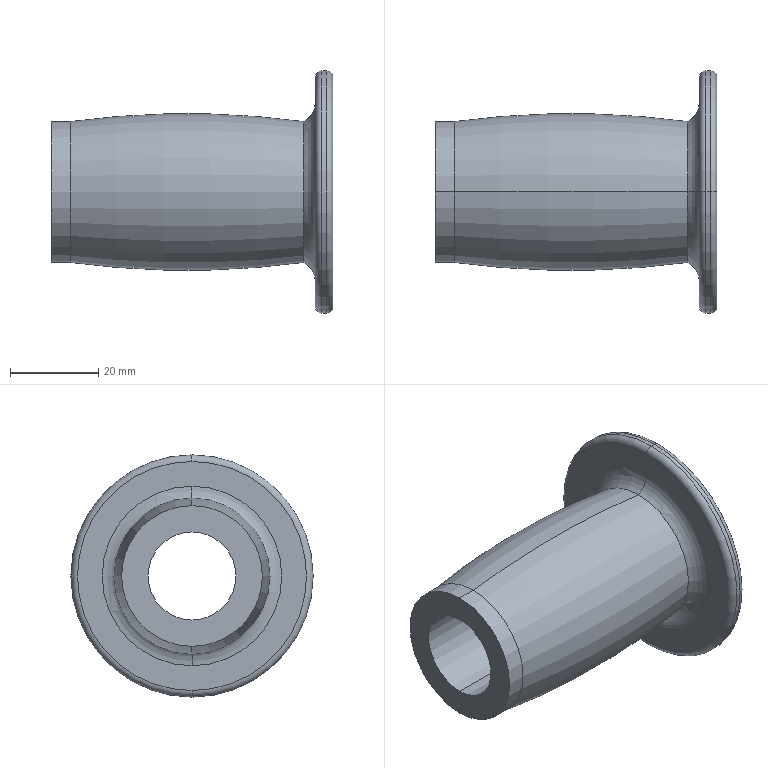Part | STEP file | Handlebar gear change grip | 1 solid | 17 faces | box 64 x 55 x 55 mm | volume 44472 mm3 | torus 6 | cylinder 6 | plane 3 | other 2 | commonest cylinder face diameters 20 x2 32 x2 55 x2
STEP:
#1=CARTESIAN_POINT('',(0.,0.,0.));
#2=DIRECTION('',(0.,0.,1.));
#3=DIRECTION('',(1.,0.,0.));
#4=AXIS2_PLACEMENT_3D('',#1,#2,#3);
#5=CARTESIAN_POINT('',(60.,0.,26.));
#6=VERTEX_POINT('',#5);
#7=CARTESIAN_POINT('',(60.,0.,-26.));
#8=VERTEX_POINT('',#7);
#9=CARTESIAN_POINT('',(60.,0.,0.));
#10=DIRECTION('',(-1.,0.,0.));
#11=DIRECTION('',(0.,0.,-1.));
#12=AXIS2_PLACEMENT_3D('',#9,#10,#11);
#13=CIRCLE('',#12,26.);
#14=CARTESIAN_POINT('',(61.5,0.,0.));
#15=DIRECTION('',(1.,0.,0.));
#16=DIRECTION('',(0.,0.,-1.));
#17=AXIS2_PLACEMENT_3D('',#14,#15,#16);
#18=TOROIDAL_SURFACE('',#17,26.,1.5);
#19=CARTESIAN_POINT('',(6.283,4.712));
#20=DIRECTION('',(-1.,0.));
#21=VECTOR('',#20,1.);
#22=LINE('',#19,#21);
#23=(GEOMETRIC_REPRESENTATION_CONTEXT(2)PARAMETRIC_REPRESENTATION_CONTEXT()REPRESENTATION_CONTEXT('',''));
#24=DEFINITIONAL_REPRESENTATION('',(#22),#23);
#25=PCURVE('',#18,#24);
#26=CARTESIAN_POINT('',(60.,0.,-16.));
#27=DIRECTION('',(1.,0.,0.));
#28=DIRECTION('',(0.,0.,-1.));
#29=AXIS2_PLACEMENT_3D('',#26,#27,#28);
#30=PLANE('',#29);
#31=CARTESIAN_POINT('',(10.,0.));
#32=CARTESIAN_POINT('',(10.,-45.033));
#33=CARTESIAN_POINT('',(-29.,-22.517));
#34=CARTESIAN_POINT('',(-68.,0.));
#35=CARTESIAN_POINT('',(-29.,22.517));
#36=CARTESIAN_POINT('',(10.,45.033));
#37=CARTESIAN_POINT('',(10.,0.));
#38=(BOUNDED_CURVE()B_SPLINE_CURVE(2,(#31,#32,#33,#34,#35,#36,#37),.UNSPECIFIED.,.T.,.F.)B_SPLINE_CURVE_WITH_KNOTS((1,2,2,2,2,1),(-2.094,0.,2.094,4.189,6.283,8.378),.UNSPECIFIED.)CURVE()GEOMETRIC_REPRESENTATION_ITEM()RATIONAL_B_SPLINE_CURVE((1.,0.5,1.,0.5,1.,0.5,1.))REPRESENTATION_ITEM(''));
#39=(GEOMETRIC_REPRESENTATION_CONTEXT(2)PARAMETRIC_REPRESENTATION_CONTEXT()REPRESENTATION_CONTEXT('',''));
#40=DEFINITIONAL_REPRESENTATION('',(#38),#39);
#41=PCURVE('',#30,#40);
#42=SURFACE_CURVE('',#13,(#25,#41),.PCURVE_S1.);
#43=EDGE_CURVE('',#6,#8,#42,.T.);
#44=ORIENTED_EDGE('',*,*,#43,.F.);
#45=CARTESIAN_POINT('',(61.5,0.,27.5));
#46=VERTEX_POINT('',#45);
#47=CARTESIAN_POINT('',(61.5,0.,26.));
#48=DIRECTION('',(0.,1.,0.));
#49=DIRECTION('',(0.,0.,1.));
#50=AXIS2_PLACEMENT_3D('',#47,#48,#49);
#51=CIRCLE('',#50,1.5);
#52=CARTESIAN_POINT('',(3.142,0.));
#53=DIRECTION('',(0.,1.));
#54=VECTOR('',#53,1.);
#55=LINE('',#52,#54);
#56=(GEOMETRIC_REPRESENTATION_CONTEXT(2)PARAMETRIC_REPRESENTATION_CONTEXT()REPRESENTATION_CONTEXT('',''));
#57=DEFINITIONAL_REPRESENTATION('',(#55),#56);
#58=PCURVE('',#18,#57);
#59=CARTESIAN_POINT('',(61.5,0.,0.));
#60=DIRECTION('',(1.,0.,0.));
#61=DIRECTION('',(0.,0.,-1.));
#62=AXIS2_PLACEMENT_3D('',#59,#60,#61);
#63=TOROIDAL_SURFACE('',#62,26.,1.5);
#64=CARTESIAN_POINT('',(3.142,0.));
#65=DIRECTION('',(0.,1.));
#66=VECTOR('',#65,1.);
#67=LINE('',#64,#66);
#68=(GEOMETRIC_REPRESENTATION_CONTEXT(2)PARAMETRIC_REPRESENTATION_CONTEXT()REPRESENTATION_CONTEXT('',''));
#69=DEFINITIONAL_REPRESENTATION('',(#67),#68);
#70=PCURVE('',#63,#69);
#71=SURFACE_CURVE('',#51,(#58,#70),.PCURVE_S1.);
#72=EDGE_CURVE('',#6,#46,#71,.T.);
#73=ORIENTED_EDGE('',*,*,#72,.T.);
#74=CARTESIAN_POINT('',(61.5,0.,-27.5));
#75=VERTEX_POINT('',#74);
#76=CARTESIAN_POINT('',(61.5,0.,0.));
#77=DIRECTION('',(1.,0.,0.));
#78=DIRECTION('',(0.,0.,-1.));
#79=AXIS2_PLACEMENT_3D('',#76,#77,#78);
#80=CIRCLE('',#79,27.5);
#81=CARTESIAN_POINT('',(0.,6.283));
#82=DIRECTION('',(1.,0.));
#83=VECTOR('',#82,1.);
#84=LINE('',#81,#83);
#85=(GEOMETRIC_REPRESENTATION_CONTEXT(2)PARAMETRIC_REPRESENTATION_CONTEXT()REPRESENTATION_CONTEXT('',''));
#86=DEFINITIONAL_REPRESENTATION('',(#84),#85);
#87=PCURVE('',#18,#86);
#88=CARTESIAN_POINT('',(64.,0.,0.));
#89=DIRECTION('',(-1.,0.,0.));
#90=DIRECTION('',(0.,0.,1.));
#91=AXIS2_PLACEMENT_3D('',#88,#89,#90);
#92=CYLINDRICAL_SURFACE('',#91,27.5);
#93=CARTESIAN_POINT('',(3.142,2.5));
#94=DIRECTION('',(-1.,0.));
#95=VECTOR('',#94,1.);
#96=LINE('',#93,#95);
#97=(GEOMETRIC_REPRESENTATION_CONTEXT(2)PARAMETRIC_REPRESENTATION_CONTEXT()REPRESENTATION_CONTEXT('',''));
#98=DEFINITIONAL_REPRESENTATION('',(#96),#97);
#99=PCURVE('',#92,#98);
#100=SURFACE_CURVE('',#80,(#87,#99),.PCURVE_S1.);
#101=EDGE_CURVE('',#75,#46,#100,.T.);
#102=ORIENTED_EDGE('',*,*,#101,.F.);
#103=CARTESIAN_POINT('',(61.5,0.,-26.));
#104=DIRECTION('',(0.,-1.,0.));
#105=DIRECTION('',(0.,0.,-1.));
#106=AXIS2_PLACEMENT_3D('',#103,#104,#105);
#107=CIRCLE('',#106,1.5);
#108=CARTESIAN_POINT('',(0.,0.));
#109=DIRECTION('',(0.,1.));
#110=VECTOR('',#109,1.);
#111=LINE('',#108,#110);
#112=(GEOMETRIC_REPRESENTATION_CONTEXT(2)PARAMETRIC_REPRESENTATION_CONTEXT()REPRESENTATION_CONTEXT('',''));
#113=DEFINITIONAL_REPRESENTATION('',(#111),#112);
#114=PCURVE('',#18,#113);
#115=CARTESIAN_POINT('',(6.283,0.));
#116=DIRECTION('',(0.,1.));
#117=VECTOR('',#116,1.);
#118=LINE('',#115,#117);
#119=(GEOMETRIC_REPRESENTATION_CONTEXT(2)PARAMETRIC_REPRESENTATION_CONTEXT()REPRESENTATION_CONTEXT('',''));
#120=DEFINITIONAL_REPRESENTATION('',(#118),#119);
#121=PCURVE('',#63,#120);
#122=SURFACE_CURVE('',#107,(#114,#121),.PCURVE_S1.);
#123=EDGE_CURVE('',#8,#75,#122,.T.);
#124=ORIENTED_EDGE('',*,*,#123,.F.);
#125=EDGE_LOOP('',(#44,#73,#102,#124));
#126=FACE_BOUND('',#125,.T.);
#127=ADVANCED_FACE('',(#126),#18,.T.);
#128=CARTESIAN_POINT('',(62.5,0.,27.5));
#129=VERTEX_POINT('',#128);
#130=CARTESIAN_POINT('',(62.5,0.,-27.5));
#131=VERTEX_POINT('',#130);
#132=CARTESIAN_POINT('',(62.5,0.,0.));
#133=DIRECTION('',(-1.,0.,0.));
#134=DIRECTION('',(0.,0.,1.));
#135=AXIS2_PLACEMENT_3D('',#132,#133,#134);
#136=CIRCLE('',#135,27.5);
#137=CARTESIAN_POINT('',(0.,1.5));
#138=DIRECTION('',(1.,0.));
#139=VECTOR('',#138,1.);
#140=LINE('',#137,#139);
#141=(GEOMETRIC_REPRESENTATION_CONTEXT(2)PARAMETRIC_REPRESENTATION_CONTEXT()REPRESENTATION_CONTEXT('',''));
#142=DEFINITIONAL_REPRESENTATION('',(#140),#141);
#143=PCURVE('',#92,#142);
#144=CARTESIAN_POINT('',(62.5,0.,0.));
#145=DIRECTION('',(-1.,0.,0.));
#146=DIRECTION('',(0.,0.,1.));
#147=AXIS2_PLACEMENT_3D('',#144,#145,#146);
#148=TOROIDAL_SURFACE('',#147,26.,1.5);
#149=CARTESIAN_POINT('',(0.,6.283));
#150=DIRECTION('',(1.,0.));
#151=VECTOR('',#150,1.);
#152=LINE('',#149,#151);
#153=(GEOMETRIC_REPRESENTATION_CONTEXT(2)PARAMETRIC_REPRESENTATION_CONTEXT()REPRESENTATION_CONTEXT('',''));
#154=DEFINITIONAL_REPRESENTATION('',(#152),#153);
#155=PCURVE('',#148,#154);
#156=SURFACE_CURVE('',#136,(#143,#155),.PCURVE_S1.);
#157=EDGE_CURVE('',#129,#131,#156,.T.);
#158=ORIENTED_EDGE('',*,*,#157,.T.);
#159=CARTESIAN_POINT('',(64.,0.,-27.5));
#160=DIRECTION('',(-1.,0.,0.));
#161=VECTOR('',#160,1.);
#162=LINE('',#159,#161);
#163=CARTESIAN_POINT('',(3.142,0.));
#164=DIRECTION('',(0.,1.));
#165=VECTOR('',#164,1.);
#166=LINE('',#163,#165);
#167=(GEOMETRIC_REPRESENTATION_CONTEXT(2)PARAMETRIC_REPRESENTATION_CONTEXT()REPRESENTATION_CONTEXT('',''));
#168=DEFINITIONAL_REPRESENTATION('',(#166),#167);
#169=PCURVE('',#92,#168);
#170=CARTESIAN_POINT('',(64.,0.,0.));
#171=DIRECTION('',(-1.,0.,0.));
#172=DIRECTION('',(0.,0.,1.));
#173=AXIS2_PLACEMENT_3D('',#170,#171,#172);
#174=CYLINDRICAL_SURFACE('',#173,27.5);
#175=CARTESIAN_POINT('',(3.142,0.));
#176=DIRECTION('',(0.,1.));
#177=VECTOR('',#176,1.);
#178=LINE('',#175,#177);
#179=(GEOMETRIC_REPRESENTATION_CONTEXT(2)PARAMETRIC_REPRESENTATION_CONTEXT()REPRESENTATION_CONTEXT('',''));
#180=DEFINITIONAL_REPRESENTATION('',(#178),#179);
#181=PCURVE('',#174,#180);
#182=SURFACE_CURVE('',#162,(#169,#181),.PCURVE_S1.);
#183=EDGE_CURVE('',#131,#75,#182,.T.);
#184=ORIENTED_EDGE('',*,*,#183,.T.);
#185=ORIENTED_EDGE('',*,*,#101,.T.);
#186=CARTESIAN_POINT('',(64.,0.,27.5));
#187=DIRECTION('',(-1.,0.,0.));
#188=VECTOR('',#187,1.);
#189=LINE('',#186,#188);
#190=CARTESIAN_POINT('',(0.,0.));
#191=DIRECTION('',(0.,1.));
#192=VECTOR('',#191,1.);
#193=LINE('',#190,#192);
#194=(GEOMETRIC_REPRESENTATION_CONTEXT(2)PARAMETRIC_REPRESENTATION_CONTEXT()REPRESENTATION_CONTEXT('',''));
#195=DEFINITIONAL_REPRESENTATION('',(#193),#194);
#196=PCURVE('',#92,#195);
#197=CARTESIAN_POINT('',(6.283,0.));
#198=DIRECTION('',(0.,1.));
#199=VECTOR('',#198,1.);
#200=LINE('',#197,#199);
#201=(GEOMETRIC_REPRESENTATION_CONTEXT(2)PARAMETRIC_REPRESENTATION_CONTEXT()REPRESENTATION_CONTEXT('',''));
#202=DEFINITIONAL_REPRESENTATION('',(#200),#201);
#203=PCURVE('',#174,#202);
#204=SURFACE_CURVE('',#189,(#196,#203),.PCURVE_S1.);
#205=EDGE_CURVE('',#129,#46,#204,.T.);
#206=ORIENTED_EDGE('',*,*,#205,.F.);
#207=EDGE_LOOP('',(#158,#184,#185,#206));
#208=FACE_BOUND('',#207,.T.);
#209=ADVANCED_FACE('',(#208),#92,.T.);
#210=ORIENTED_EDGE('',*,*,#183,.F.);
#211=CARTESIAN_POINT('',(62.5,0.,0.));
#212=DIRECTION('',(-1.,0.,0.));
#213=DIRECTION('',(0.,0.,1.));
#214=AXIS2_PLACEMENT_3D('',#211,#212,#213);
#215=CIRCLE('',#214,27.5);
#216=CARTESIAN_POINT('',(0.,1.5));
#217=DIRECTION('',(1.,0.));
#218=VECTOR('',#217,1.);
#219=LINE('',#216,#218);
#220=(GEOMETRIC_REPRESENTATION_CONTEXT(2)PARAMETRIC_REPRESENTATION_CONTEXT()REPRESENTATION_CONTEXT('',''));
#221=DEFINITIONAL_REPRESENTATION('',(#219),#220);
#222=PCURVE('',#174,#221);
#223=CARTESIAN_POINT('',(62.5,0.,0.));
#224=DIRECTION('',(-1.,0.,0.));
#225=DIRECTION('',(0.,0.,1.));
#226=AXIS2_PLACEMENT_3D('',#223,#224,#225);
#227=TOROIDAL_SURFACE('',#226,26.,1.5);
#228=CARTESIAN_POINT('',(0.,6.283));
#229=DIRECTION('',(1.,0.));
#230=VECTOR('',#229,1.);
#231=LINE('',#228,#230);
#232=(GEOMETRIC_REPRESENTATION_CONTEXT(2)PARAMETRIC_REPRESENTATION_CONTEXT()REPRESENTATION_CONTEXT('',''));
#233=DEFINITIONAL_REPRESENTATION('',(#231),#232);
#234=PCURVE('',#227,#233);
#235=SURFACE_CURVE('',#215,(#222,#234),.PCURVE_S1.);
#236=EDGE_CURVE('',#131,#129,#235,.T.);
#237=ORIENTED_EDGE('',*,*,#236,.T.);
#238=ORIENTED_EDGE('',*,*,#205,.T.);
#239=CARTESIAN_POINT('',(61.5,0.,0.));
#240=DIRECTION('',(1.,0.,0.));
#241=DIRECTION('',(0.,0.,-1.));
#242=AXIS2_PLACEMENT_3D('',#239,#240,#241);
#243=CIRCLE('',#242,27.5);
#244=CARTESIAN_POINT('',(9.425,2.5));
#245=DIRECTION('',(-1.,0.));
#246=VECTOR('',#245,1.);
#247=LINE('',#244,#246);
#248=(GEOMETRIC_REPRESENTATION_CONTEXT(2)PARAMETRIC_REPRESENTATION_CONTEXT()REPRESENTATION_CONTEXT('',''));
#249=DEFINITIONAL_REPRESENTATION('',(#247),#248);
#250=PCURVE('',#174,#249);
#251=CARTESIAN_POINT('',(0.,6.283));
#252=DIRECTION('',(1.,0.));
#253=VECTOR('',#252,1.);
#254=LINE('',#251,#253);
#255=(GEOMETRIC_REPRESENTATION_CONTEXT(2)PARAMETRIC_REPRESENTATION_CONTEXT()REPRESENTATION_CONTEXT('',''));
#256=DEFINITIONAL_REPRESENTATION('',(#254),#255);
#257=PCURVE('',#63,#256);
#258=SURFACE_CURVE('',#243,(#250,#257),.PCURVE_S1.);
#259=EDGE_CURVE('',#46,#75,#258,.T.);
#260=ORIENTED_EDGE('',*,*,#259,.T.);
#261=EDGE_LOOP('',(#210,#237,#238,#260));
#262=FACE_BOUND('',#261,.T.);
#263=ADVANCED_FACE('',(#262),#174,.T.);
#264=CARTESIAN_POINT('',(64.,0.,-26.));
#265=VERTEX_POINT('',#264);
#266=CARTESIAN_POINT('',(62.5,0.,-26.));
#267=DIRECTION('',(0.,1.,0.));
#268=DIRECTION('',(0.,0.,1.));
#269=AXIS2_PLACEMENT_3D('',#266,#267,#268);
#270=CIRCLE('',#269,1.5);
#271=CARTESIAN_POINT('',(3.142,3.142));
#272=DIRECTION('',(0.,1.));
#273=VECTOR('',#272,1.);
#274=LINE('',#271,#273);
#275=(GEOMETRIC_REPRESENTATION_CONTEXT(2)PARAMETRIC_REPRESENTATION_CONTEXT()REPRESENTATION_CONTEXT('',''));
#276=DEFINITIONAL_REPRESENTATION('',(#274),#275);
#277=PCURVE('',#227,#276);
#278=CARTESIAN_POINT('',(3.142,3.142));
#279=DIRECTION('',(0.,1.));
#280=VECTOR('',#279,1.);
#281=LINE('',#278,#280);
#282=(GEOMETRIC_REPRESENTATION_CONTEXT(2)PARAMETRIC_REPRESENTATION_CONTEXT()REPRESENTATION_CONTEXT('',''));
#283=DEFINITIONAL_REPRESENTATION('',(#281),#282);
#284=PCURVE('',#148,#283);
#285=SURFACE_CURVE('',#270,(#277,#284),.PCURVE_S1.);
#286=EDGE_CURVE('',#265,#131,#285,.T.);
#287=ORIENTED_EDGE('',*,*,#286,.F.);
#288=CARTESIAN_POINT('',(64.,0.,26.));
#289=VERTEX_POINT('',#288);
#290=CARTESIAN_POINT('',(64.,0.,0.));
#291=DIRECTION('',(1.,0.,0.));
#292=DIRECTION('',(0.,0.,1.));
#293=AXIS2_PLACEMENT_3D('',#290,#291,#292);
#294=CIRCLE('',#293,26.);
#295=CARTESIAN_POINT('',(6.283,4.712));
#296=DIRECTION('',(-1.,0.));
#297=VECTOR('',#296,1.);
#298=LINE('',#295,#297);
#299=(GEOMETRIC_REPRESENTATION_CONTEXT(2)PARAMETRIC_REPRESENTATION_CONTEXT()REPRESENTATION_CONTEXT('',''));
#300=DEFINITIONAL_REPRESENTATION('',(#298),#299);
#301=PCURVE('',#227,#300);
#302=CARTESIAN_POINT('',(64.,0.,-10.));
#303=DIRECTION('',(-1.,0.,0.));
#304=DIRECTION('',(0.,0.,1.));
#305=AXIS2_PLACEMENT_3D('',#302,#303,#304);
#306=PLANE('',#305);
#307=CARTESIAN_POINT('',(36.,0.));
#308=CARTESIAN_POINT('',(36.,-45.033));
#309=CARTESIAN_POINT('',(-3.,-22.517));
#310=CARTESIAN_POINT('',(-42.,0.));
#311=CARTESIAN_POINT('',(-3.,22.517));
#312=CARTESIAN_POINT('',(36.,45.033));
#313=CARTESIAN_POINT('',(36.,0.));
#314=(BOUNDED_CURVE()B_SPLINE_CURVE(2,(#307,#308,#309,#310,#311,#312,#313),.UNSPECIFIED.,.T.,.F.)B_SPLINE_CURVE_WITH_KNOTS((1,2,2,2,2,1),(-2.094,0.,2.094,4.189,6.283,8.378),.UNSPECIFIED.)CURVE()GEOMETRIC_REPRESENTATION_ITEM()RATIONAL_B_SPLINE_CURVE((1.,0.5,1.,0.5,1.,0.5,1.))REPRESENTATION_ITEM(''));
#315=(GEOMETRIC_REPRESENTATION_CONTEXT(2)PARAMETRIC_REPRESENTATION_CONTEXT()REPRESENTATION_CONTEXT('',''));
#316=DEFINITIONAL_REPRESENTATION('',(#314),#315);
#317=PCURVE('',#306,#316);
#318=SURFACE_CURVE('',#294,(#301,#317),.PCURVE_S1.);
#319=EDGE_CURVE('',#289,#265,#318,.T.);
#320=ORIENTED_EDGE('',*,*,#319,.F.);
#321=CARTESIAN_POINT('',(62.5,0.,26.));
#322=DIRECTION('',(0.,-1.,0.));
#323=DIRECTION('',(0.,0.,-1.));
#324=AXIS2_PLACEMENT_3D('',#321,#322,#323);
#325=CIRCLE('',#324,1.5);
#326=CARTESIAN_POINT('',(6.283,3.142));
#327=DIRECTION('',(0.,1.));
#328=VECTOR('',#327,1.);
#329=LINE('',#326,#328);
#330=(GEOMETRIC_REPRESENTATION_CONTEXT(2)PARAMETRIC_REPRESENTATION_CONTEXT()REPRESENTATION_CONTEXT('',''));
#331=DEFINITIONAL_REPRESENTATION('',(#329),#330);
#332=PCURVE('',#227,#331);
#333=CARTESIAN_POINT('',(0.,3.142));
#334=DIRECTION('',(0.,1.));
#335=VECTOR('',#334,1.);
#336=LINE('',#333,#335);
#337=(GEOMETRIC_REPRESENTATION_CONTEXT(2)PARAMETRIC_REPRESENTATION_CONTEXT()REPRESENTATION_CONTEXT('',''));
#338=DEFINITIONAL_REPRESENTATION('',(#336),#337);
#339=PCURVE('',#148,#338);
#340=SURFACE_CURVE('',#325,(#332,#339),.PCURVE_S1.);
#341=EDGE_CURVE('',#289,#129,#340,.T.);
#342=ORIENTED_EDGE('',*,*,#341,.T.);
#343=ORIENTED_EDGE('',*,*,#236,.F.);
#344=EDGE_LOOP('',(#287,#320,#342,#343));
#345=FACE_BOUND('',#344,.T.);
#346=ADVANCED_FACE('',(#345),#227,.T.);
#347=ORIENTED_EDGE('',*,*,#319,.T.);
#348=CARTESIAN_POINT('',(64.,0.,0.));
#349=DIRECTION('',(1.,0.,0.));
#350=DIRECTION('',(0.,0.,1.));
#351=AXIS2_PLACEMENT_3D('',#348,#349,#350);
#352=CIRCLE('',#351,26.);
#353=CARTESIAN_POINT('',(36.,0.));
#354=CARTESIAN_POINT('',(36.,-45.033));
#355=CARTESIAN_POINT('',(-3.,-22.517));
#356=CARTESIAN_POINT('',(-42.,0.));
#357=CARTESIAN_POINT('',(-3.,22.517));
#358=CARTESIAN_POINT('',(36.,45.033));
#359=CARTESIAN_POINT('',(36.,0.));
#360=(BOUNDED_CURVE()B_SPLINE_CURVE(2,(#353,#354,#355,#356,#357,#358,#359),.UNSPECIFIED.,.T.,.F.)B_SPLINE_CURVE_WITH_KNOTS((1,2,2,2,2,1),(-2.094,0.,2.094,4.189,6.283,8.378),.UNSPECIFIED.)CURVE()GEOMETRIC_REPRESENTATION_ITEM()RATIONAL_B_SPLINE_CURVE((1.,0.5,1.,0.5,1.,0.5,1.))REPRESENTATION_ITEM(''));
#361=(GEOMETRIC_REPRESENTATION_CONTEXT(2)PARAMETRIC_REPRESENTATION_CONTEXT()REPRESENTATION_CONTEXT('',''));
#362=DEFINITIONAL_REPRESENTATION('',(#360),#361);
#363=PCURVE('',#306,#362);
#364=CARTESIAN_POINT('',(6.283,4.712));
#365=DIRECTION('',(-1.,0.));
#366=VECTOR('',#365,1.);
#367=LINE('',#364,#366);
#368=(GEOMETRIC_REPRESENTATION_CONTEXT(2)PARAMETRIC_REPRESENTATION_CONTEXT()REPRESENTATION_CONTEXT('',''));
#369=DEFINITIONAL_REPRESENTATION('',(#367),#368);
#370=PCURVE('',#148,#369);
#371=SURFACE_CURVE('',#352,(#363,#370),.PCURVE_S1.);
#372=EDGE_CURVE('',#265,#289,#371,.T.);
#373=ORIENTED_EDGE('',*,*,#372,.T.);
#374=EDGE_LOOP('',(#347,#373));
#375=FACE_BOUND('',#374,.T.);
#376=CARTESIAN_POINT('',(64.,0.,10.));
#377=VERTEX_POINT('',#376);
#378=CARTESIAN_POINT('',(64.,0.,-10.));
#379=VERTEX_POINT('',#378);
#380=CARTESIAN_POINT('',(64.,0.,0.));
#381=DIRECTION('',(-1.,0.,0.));
#382=DIRECTION('',(0.,0.,1.));
#383=AXIS2_PLACEMENT_3D('',#380,#381,#382);
#384=CIRCLE('',#383,10.);
#385=CARTESIAN_POINT('',(10.,0.));
#386=DIRECTION('',(1.,0.));
#387=AXIS2_PLACEMENT_2D('',#385,#386);
#388=CIRCLE('',#387,10.);
#389=(GEOMETRIC_REPRESENTATION_CONTEXT(2)PARAMETRIC_REPRESENTATION_CONTEXT()REPRESENTATION_CONTEXT('',''));
#390=DEFINITIONAL_REPRESENTATION('',(#388),#389);
#391=PCURVE('',#306,#390);
#392=CARTESIAN_POINT('',(64.,0.,0.));
#393=DIRECTION('',(-1.,0.,0.));
#394=DIRECTION('',(0.,0.,1.));
#395=AXIS2_PLACEMENT_3D('',#392,#393,#394);
#396=CYLINDRICAL_SURFACE('',#395,10.);
#397=CARTESIAN_POINT('',(0.,0.));
#398=DIRECTION('',(1.,0.));
#399=VECTOR('',#398,1.);
#400=LINE('',#397,#399);
#401=(GEOMETRIC_REPRESENTATION_CONTEXT(2)PARAMETRIC_REPRESENTATION_CONTEXT()REPRESENTATION_CONTEXT('',''));
#402=DEFINITIONAL_REPRESENTATION('',(#400),#401);
#403=PCURVE('',#396,#402);
#404=SURFACE_CURVE('',#384,(#391,#403),.PCURVE_S1.);
#405=EDGE_CURVE('',#377,#379,#404,.T.);
#406=ORIENTED_EDGE('',*,*,#405,.T.);
#407=CARTESIAN_POINT('',(64.,0.,0.));
#408=DIRECTION('',(-1.,0.,0.));
#409=DIRECTION('',(0.,0.,1.));
#410=AXIS2_PLACEMENT_3D('',#407,#408,#409);
#411=CIRCLE('',#410,10.);
#412=CARTESIAN_POINT('',(10.,0.));
#413=DIRECTION('',(1.,0.));
#414=AXIS2_PLACEMENT_2D('',#412,#413);
#415=CIRCLE('',#414,10.);
#416=(GEOMETRIC_REPRESENTATION_CONTEXT(2)PARAMETRIC_REPRESENTATION_CONTEXT()REPRESENTATION_CONTEXT('',''));
#417=DEFINITIONAL_REPRESENTATION('',(#415),#416);
#418=PCURVE('',#306,#417);
#419=CARTESIAN_POINT('',(64.,0.,0.));
#420=DIRECTION('',(-1.,0.,0.));
#421=DIRECTION('',(0.,0.,1.));
#422=AXIS2_PLACEMENT_3D('',#419,#420,#421);
#423=CYLINDRICAL_SURFACE('',#422,10.);
#424=CARTESIAN_POINT('',(0.,0.));
#425=DIRECTION('',(1.,0.));
#426=VECTOR('',#425,1.);
#427=LINE('',#424,#426);
#428=(GEOMETRIC_REPRESENTATION_CONTEXT(2)PARAMETRIC_REPRESENTATION_CONTEXT()REPRESENTATION_CONTEXT('',''));
#429=DEFINITIONAL_REPRESENTATION('',(#427),#428);
#430=PCURVE('',#423,#429);
#431=SURFACE_CURVE('',#411,(#418,#430),.PCURVE_S1.);
#432=EDGE_CURVE('',#379,#377,#431,.T.);
#433=ORIENTED_EDGE('',*,*,#432,.T.);
#434=EDGE_LOOP('',(#406,#433));
#435=FACE_BOUND('',#434,.T.);
#436=ADVANCED_FACE('',(#375,#435),#306,.F.);
#437=CARTESIAN_POINT('',(0.,0.,10.));
#438=VERTEX_POINT('',#437);
#439=CARTESIAN_POINT('',(64.,0.,10.));
#440=DIRECTION('',(-1.,0.,0.));
#441=VECTOR('',#440,1.);
#442=LINE('',#439,#441);
#443=CARTESIAN_POINT('',(6.283,0.));
#444=DIRECTION('',(0.,1.));
#445=VECTOR('',#444,1.);
#446=LINE('',#443,#445);
#447=(GEOMETRIC_REPRESENTATION_CONTEXT(2)PARAMETRIC_REPRESENTATION_CONTEXT()REPRESENTATION_CONTEXT('',''));
#448=DEFINITIONAL_REPRESENTATION('',(#446),#447);
#449=PCURVE('',#423,#448);
#450=CARTESIAN_POINT('',(0.,0.));
#451=DIRECTION('',(0.,1.));
#452=VECTOR('',#451,1.);
#453=LINE('',#450,#452);
#454=(GEOMETRIC_REPRESENTATION_CONTEXT(2)PARAMETRIC_REPRESENTATION_CONTEXT()REPRESENTATION_CONTEXT('',''));
#455=DEFINITIONAL_REPRESENTATION('',(#453),#454);
#456=PCURVE('',#396,#455);
#457=SURFACE_CURVE('',#442,(#449,#456),.PCURVE_S1.);
#458=EDGE_CURVE('',#377,#438,#457,.T.);
#459=ORIENTED_EDGE('',*,*,#458,.T.);
#460=CARTESIAN_POINT('',(0.,0.,-10.));
#461=VERTEX_POINT('',#460);
#462=CARTESIAN_POINT('',(0.,0.,0.));
#463=DIRECTION('',(-1.,0.,0.));
#464=DIRECTION('',(0.,0.,1.));
#465=AXIS2_PLACEMENT_3D('',#462,#463,#464);
#466=CIRCLE('',#465,10.);
#467=CARTESIAN_POINT('',(0.,64.));
#468=DIRECTION('',(1.,0.));
#469=VECTOR('',#468,1.);
#470=LINE('',#467,#469);
#471=(GEOMETRIC_REPRESENTATION_CONTEXT(2)PARAMETRIC_REPRESENTATION_CONTEXT()REPRESENTATION_CONTEXT('',''));
#472=DEFINITIONAL_REPRESENTATION('',(#470),#471);
#473=PCURVE('',#423,#472);
#474=CARTESIAN_POINT('',(0.,0.,-10.));
#475=DIRECTION('',(1.,0.,0.));
#476=DIRECTION('',(0.,0.,-1.));
#477=AXIS2_PLACEMENT_3D('',#474,#475,#476);
#478=PLANE('',#477);
#479=CARTESIAN_POINT('',(-20.,0.));
#480=CARTESIAN_POINT('',(-20.,17.321));
#481=CARTESIAN_POINT('',(-5.,8.66));
#482=CARTESIAN_POINT('',(10.,0.));
#483=CARTESIAN_POINT('',(-5.,-8.66));
#484=CARTESIAN_POINT('',(-20.,-17.321));
#485=CARTESIAN_POINT('',(-20.,0.));
#486=(BOUNDED_CURVE()B_SPLINE_CURVE(2,(#479,#480,#481,#482,#483,#484,#485),.UNSPECIFIED.,.T.,.F.)B_SPLINE_CURVE_WITH_KNOTS((1,2,2,2,2,1),(-2.094,0.,2.094,4.189,6.283,8.378),.UNSPECIFIED.)CURVE()GEOMETRIC_REPRESENTATION_ITEM()RATIONAL_B_SPLINE_CURVE((1.,0.5,1.,0.5,1.,0.5,1.))REPRESENTATION_ITEM(''));
#487=(GEOMETRIC_REPRESENTATION_CONTEXT(2)PARAMETRIC_REPRESENTATION_CONTEXT()REPRESENTATION_CONTEXT('',''));
#488=DEFINITIONAL_REPRESENTATION('',(#486),#487);
#489=PCURVE('',#478,#488);
#490=SURFACE_CURVE('',#466,(#473,#489),.PCURVE_S1.);
#491=EDGE_CURVE('',#461,#438,#490,.T.);
#492=ORIENTED_EDGE('',*,*,#491,.F.);
#493=CARTESIAN_POINT('',(64.,0.,-10.));
#494=DIRECTION('',(-1.,0.,0.));
#495=VECTOR('',#494,1.);
#496=LINE('',#493,#495);
#497=CARTESIAN_POINT('',(3.142,0.));
#498=DIRECTION('',(0.,1.));
#499=VECTOR('',#498,1.);
#500=LINE('',#497,#499);
#501=(GEOMETRIC_REPRESENTATION_CONTEXT(2)PARAMETRIC_REPRESENTATION_CONTEXT()REPRESENTATION_CONTEXT('',''));
#502=DEFINITIONAL_REPRESENTATION('',(#500),#501);
#503=PCURVE('',#423,#502);
#504=CARTESIAN_POINT('',(3.142,0.));
#505=DIRECTION('',(0.,1.));
#506=VECTOR('',#505,1.);
#507=LINE('',#504,#506);
#508=(GEOMETRIC_REPRESENTATION_CONTEXT(2)PARAMETRIC_REPRESENTATION_CONTEXT()REPRESENTATION_CONTEXT('',''));
#509=DEFINITIONAL_REPRESENTATION('',(#507),#508);
#510=PCURVE('',#396,#509);
#511=SURFACE_CURVE('',#496,(#503,#510),.PCURVE_S1.);
#512=EDGE_CURVE('',#379,#461,#511,.T.);
#513=ORIENTED_EDGE('',*,*,#512,.F.);
#514=ORIENTED_EDGE('',*,*,#432,.T.);
#515=EDGE_LOOP('',(#459,#492,#513,#514));
#516=FACE_BOUND('',#515,.F.);
#517=ADVANCED_FACE('',(#516),#423,.F.);
#518=CARTESIAN_POINT('',(0.,0.,0.));
#519=DIRECTION('',(-1.,0.,0.));
#520=DIRECTION('',(0.,0.,1.));
#521=AXIS2_PLACEMENT_3D('',#518,#519,#520);
#522=CIRCLE('',#521,10.);
#523=CARTESIAN_POINT('',(-20.,0.));
#524=CARTESIAN_POINT('',(-20.,17.321));
#525=CARTESIAN_POINT('',(-5.,8.66));
#526=CARTESIAN_POINT('',(10.,0.));
#527=CARTESIAN_POINT('',(-5.,-8.66));
#528=CARTESIAN_POINT('',(-20.,-17.321));
#529=CARTESIAN_POINT('',(-20.,0.));
#530=(BOUNDED_CURVE()B_SPLINE_CURVE(2,(#523,#524,#525,#526,#527,#528,#529),.UNSPECIFIED.,.T.,.F.)B_SPLINE_CURVE_WITH_KNOTS((1,2,2,2,2,1),(-2.094,0.,2.094,4.189,6.283,8.378),.UNSPECIFIED.)CURVE()GEOMETRIC_REPRESENTATION_ITEM()RATIONAL_B_SPLINE_CURVE((1.,0.5,1.,0.5,1.,0.5,1.))REPRESENTATION_ITEM(''));
#531=(GEOMETRIC_REPRESENTATION_CONTEXT(2)PARAMETRIC_REPRESENTATION_CONTEXT()REPRESENTATION_CONTEXT('',''));
#532=DEFINITIONAL_REPRESENTATION('',(#530),#531);
#533=PCURVE('',#478,#532);
#534=CARTESIAN_POINT('',(0.,64.));
#535=DIRECTION('',(1.,0.));
#536=VECTOR('',#535,1.);
#537=LINE('',#534,#536);
#538=(GEOMETRIC_REPRESENTATION_CONTEXT(2)PARAMETRIC_REPRESENTATION_CONTEXT()REPRESENTATION_CONTEXT('',''));
#539=DEFINITIONAL_REPRESENTATION('',(#537),#538);
#540=PCURVE('',#396,#539);
#541=SURFACE_CURVE('',#522,(#533,#540),.PCURVE_S1.);
#542=EDGE_CURVE('',#438,#461,#541,.T.);
#543=ORIENTED_EDGE('',*,*,#542,.F.);
#544=ORIENTED_EDGE('',*,*,#491,.F.);
#545=EDGE_LOOP('',(#543,#544));
#546=FACE_BOUND('',#545,.T.);
#547=CARTESIAN_POINT('',(0.,0.,16.));
#548=VERTEX_POINT('',#547);
#549=CARTESIAN_POINT('',(0.,0.,-16.));
#550=VERTEX_POINT('',#549);
#551=CARTESIAN_POINT('',(0.,0.,0.));
#552=DIRECTION('',(-1.,0.,0.));
#553=DIRECTION('',(0.,0.,1.));
#554=AXIS2_PLACEMENT_3D('',#551,#552,#553);
#555=CIRCLE('',#554,16.);
#556=CARTESIAN_POINT('',(-26.,0.));
#557=CARTESIAN_POINT('',(-26.,27.713));
#558=CARTESIAN_POINT('',(-2.,13.856));
#559=CARTESIAN_POINT('',(22.,0.));
#560=CARTESIAN_POINT('',(-2.,-13.856));
#561=CARTESIAN_POINT('',(-26.,-27.713));
#562=CARTESIAN_POINT('',(-26.,0.));
#563=(BOUNDED_CURVE()B_SPLINE_CURVE(2,(#556,#557,#558,#559,#560,#561,#562),.UNSPECIFIED.,.T.,.F.)B_SPLINE_CURVE_WITH_KNOTS((1,2,2,2,2,1),(-2.094,0.,2.094,4.189,6.283,8.378),.UNSPECIFIED.)CURVE()GEOMETRIC_REPRESENTATION_ITEM()RATIONAL_B_SPLINE_CURVE((1.,0.5,1.,0.5,1.,0.5,1.))REPRESENTATION_ITEM(''));
#564=(GEOMETRIC_REPRESENTATION_CONTEXT(2)PARAMETRIC_REPRESENTATION_CONTEXT()REPRESENTATION_CONTEXT('',''));
#565=DEFINITIONAL_REPRESENTATION('',(#563),#564);
#566=PCURVE('',#478,#565);
#567=CARTESIAN_POINT('',(64.,0.,0.));
#568=DIRECTION('',(-1.,0.,0.));
#569=DIRECTION('',(0.,0.,1.));
#570=AXIS2_PLACEMENT_3D('',#567,#568,#569);
#571=CYLINDRICAL_SURFACE('',#570,16.);
#572=CARTESIAN_POINT('',(0.,64.));
#573=DIRECTION('',(1.,0.));
#574=VECTOR('',#573,1.);
#575=LINE('',#572,#574);
#576=(GEOMETRIC_REPRESENTATION_CONTEXT(2)PARAMETRIC_REPRESENTATION_CONTEXT()REPRESENTATION_CONTEXT('',''));
#577=DEFINITIONAL_REPRESENTATION('',(#575),#576);
#578=PCURVE('',#571,#577);
#579=SURFACE_CURVE('',#555,(#566,#578),.PCURVE_S1.);
#580=EDGE_CURVE('',#548,#550,#579,.T.);
#581=ORIENTED_EDGE('',*,*,#580,.T.);
#582=CARTESIAN_POINT('',(0.,0.,0.));
#583=DIRECTION('',(-1.,0.,0.));
#584=DIRECTION('',(0.,0.,1.));
#585=AXIS2_PLACEMENT_3D('',#582,#583,#584);
#586=CIRCLE('',#585,16.);
#587=CARTESIAN_POINT('',(-26.,0.));
#588=CARTESIAN_POINT('',(-26.,27.713));
#589=CARTESIAN_POINT('',(-2.,13.856));
#590=CARTESIAN_POINT('',(22.,0.));
#591=CARTESIAN_POINT('',(-2.,-13.856));
#592=CARTESIAN_POINT('',(-26.,-27.713));
#593=CARTESIAN_POINT('',(-26.,0.));
#594=(BOUNDED_CURVE()B_SPLINE_CURVE(2,(#587,#588,#589,#590,#591,#592,#593),.UNSPECIFIED.,.T.,.F.)B_SPLINE_CURVE_WITH_KNOTS((1,2,2,2,2,1),(-2.094,0.,2.094,4.189,6.283,8.378),.UNSPECIFIED.)CURVE()GEOMETRIC_REPRESENTATION_ITEM()RATIONAL_B_SPLINE_CURVE((1.,0.5,1.,0.5,1.,0.5,1.))REPRESENTATION_ITEM(''));
#595=(GEOMETRIC_REPRESENTATION_CONTEXT(2)PARAMETRIC_REPRESENTATION_CONTEXT()REPRESENTATION_CONTEXT('',''));
#596=DEFINITIONAL_REPRESENTATION('',(#594),#595);
#597=PCURVE('',#478,#596);
#598=CARTESIAN_POINT('',(64.,0.,0.));
#599=DIRECTION('',(-1.,0.,0.));
#600=DIRECTION('',(0.,0.,1.));
#601=AXIS2_PLACEMENT_3D('',#598,#599,#600);
#602=CYLINDRICAL_SURFACE('',#601,16.);
#603=CARTESIAN_POINT('',(0.,64.));
#604=DIRECTION('',(1.,0.));
#605=VECTOR('',#604,1.);
#606=LINE('',#603,#605);
#607=(GEOMETRIC_REPRESENTATION_CONTEXT(2)PARAMETRIC_REPRESENTATION_CONTEXT()REPRESENTATION_CONTEXT('',''));
#608=DEFINITIONAL_REPRESENTATION('',(#606),#607);
#609=PCURVE('',#602,#608);
#610=SURFACE_CURVE('',#586,(#597,#609),.PCURVE_S1.);
#611=EDGE_CURVE('',#550,#548,#610,.T.);
#612=ORIENTED_EDGE('',*,*,#611,.T.);
#613=EDGE_LOOP('',(#581,#612));
#614=FACE_BOUND('',#613,.T.);
#615=ADVANCED_FACE('',(#546,#614),#478,.F.);
#616=CARTESIAN_POINT('',(4.315,0.,-16.));
#617=VERTEX_POINT('',#616);
#618=CARTESIAN_POINT('',(64.,0.,-16.));
#619=DIRECTION('',(-1.,0.,0.));
#620=VECTOR('',#619,1.);
#621=LINE('',#618,#620);
#622=CARTESIAN_POINT('',(3.142,0.));
#623=DIRECTION('',(0.,1.));
#624=VECTOR('',#623,1.);
#625=LINE('',#622,#624);
#626=(GEOMETRIC_REPRESENTATION_CONTEXT(2)PARAMETRIC_REPRESENTATION_CONTEXT()REPRESENTATION_CONTEXT('',''));
#627=DEFINITIONAL_REPRESENTATION('',(#625),#626);
#628=PCURVE('',#602,#627);
#629=CARTESIAN_POINT('',(3.142,0.));
#630=DIRECTION('',(0.,1.));
#631=VECTOR('',#630,1.);
#632=LINE('',#629,#631);
#633=(GEOMETRIC_REPRESENTATION_CONTEXT(2)PARAMETRIC_REPRESENTATION_CONTEXT()REPRESENTATION_CONTEXT('',''));
#634=DEFINITIONAL_REPRESENTATION('',(#632),#633);
#635=PCURVE('',#571,#634);
#636=SURFACE_CURVE('',#621,(#628,#635),.PCURVE_S1.);
#637=EDGE_CURVE('',#617,#550,#636,.T.);
#638=ORIENTED_EDGE('',*,*,#637,.F.);
#639=CARTESIAN_POINT('',(4.315,0.,16.));
#640=VERTEX_POINT('',#639);
#641=CARTESIAN_POINT('',(4.315,0.,0.));
#642=DIRECTION('',(-1.,0.,0.));
#643=DIRECTION('',(0.,0.,1.));
#644=AXIS2_PLACEMENT_3D('',#641,#642,#643);
#645=CIRCLE('',#644,16.);
#646=CARTESIAN_POINT('',(0.,59.685));
#647=DIRECTION('',(1.,0.));
#648=VECTOR('',#647,1.);
#649=LINE('',#646,#648);
#650=(GEOMETRIC_REPRESENTATION_CONTEXT(2)PARAMETRIC_REPRESENTATION_CONTEXT()REPRESENTATION_CONTEXT('',''));
#651=DEFINITIONAL_REPRESENTATION('',(#649),#650);
#652=PCURVE('',#602,#651);
#653=CARTESIAN_POINT('',(4.315,0.,-16.));
#654=CARTESIAN_POINT('',(14.868,0.,-17.424));
#655=CARTESIAN_POINT('',(25.518,0.,-18.141));
#656=CARTESIAN_POINT('',(36.199,0.,-18.141));
#657=CARTESIAN_POINT('',(46.848,0.,-17.424));
#658=CARTESIAN_POINT('',(57.402,0.,-16.));
#659=B_SPLINE_CURVE_WITH_KNOTS('',5,(#653,#654,#655,#656,#657,#658),.UNSPECIFIED.,.F.,.F.,(6,6),(3.007,3.276),.PIECEWISE_BEZIER_KNOTS.);
#660=CARTESIAN_POINT('',(30.858,0.,0.));
#661=DIRECTION('',(-1.,0.,0.));
#662=AXIS1_PLACEMENT('',#660,#661);
#663=SURFACE_OF_REVOLUTION('',#659,#662);
#664=CARTESIAN_POINT('',(-3.142,3.007));
#665=DIRECTION('',(1.,0.));
#666=VECTOR('',#665,1.);
#667=LINE('',#664,#666);
#668=(GEOMETRIC_REPRESENTATION_CONTEXT(2)PARAMETRIC_REPRESENTATION_CONTEXT()REPRESENTATION_CONTEXT('',''));
#669=DEFINITIONAL_REPRESENTATION('',(#667),#668);
#670=PCURVE('',#663,#669);
#671=SURFACE_CURVE('',#645,(#652,#670),.PCURVE_S1.);
#672=EDGE_CURVE('',#617,#640,#671,.T.);
#673=ORIENTED_EDGE('',*,*,#672,.T.);
#674=CARTESIAN_POINT('',(64.,0.,16.));
#675=DIRECTION('',(-1.,0.,0.));
#676=VECTOR('',#675,1.);
#677=LINE('',#674,#676);
#678=CARTESIAN_POINT('',(6.283,0.));
#679=DIRECTION('',(0.,1.));
#680=VECTOR('',#679,1.);
#681=LINE('',#678,#680);
#682=(GEOMETRIC_REPRESENTATION_CONTEXT(2)PARAMETRIC_REPRESENTATION_CONTEXT()REPRESENTATION_CONTEXT('',''));
#683=DEFINITIONAL_REPRESENTATION('',(#681),#682);
#684=PCURVE('',#602,#683);
#685=CARTESIAN_POINT('',(0.,0.));
#686=DIRECTION('',(0.,1.));
#687=VECTOR('',#686,1.);
#688=LINE('',#685,#687);
#689=(GEOMETRIC_REPRESENTATION_CONTEXT(2)PARAMETRIC_REPRESENTATION_CONTEXT()REPRESENTATION_CONTEXT('',''));
#690=DEFINITIONAL_REPRESENTATION('',(#688),#689);
#691=PCURVE('',#571,#690);
#692=SURFACE_CURVE('',#677,(#684,#691),.PCURVE_S1.);
#693=EDGE_CURVE('',#640,#548,#692,.T.);
#694=ORIENTED_EDGE('',*,*,#693,.T.);
#695=ORIENTED_EDGE('',*,*,#611,.F.);
#696=EDGE_LOOP('',(#638,#673,#694,#695));
#697=FACE_BOUND('',#696,.T.);
#698=ADVANCED_FACE('',(#697),#602,.T.);
#699=ORIENTED_EDGE('',*,*,#672,.T.);
#700=CARTESIAN_POINT('',(57.402,0.,16.));
#701=VERTEX_POINT('',#700);
#702=CARTESIAN_POINT('',(30.858,0.,-180.672));
#703=DIRECTION('',(0.,-1.,0.));
#704=DIRECTION('',(0.,0.,-1.));
#705=AXIS2_PLACEMENT_3D('',#702,#703,#704);
#706=CIRCLE('',#705,198.455);
#707=CARTESIAN_POINT('',(3.142,6.283));
#708=DIRECTION('',(0.,-1.));
#709=VECTOR('',#708,1.);
#710=LINE('',#707,#709);
#711=(GEOMETRIC_REPRESENTATION_CONTEXT(2)PARAMETRIC_REPRESENTATION_CONTEXT()REPRESENTATION_CONTEXT('',''));
#712=DEFINITIONAL_REPRESENTATION('',(#710),#711);
#713=PCURVE('',#663,#712);
#714=CARTESIAN_POINT('',(4.315,0.,-16.));
#715=CARTESIAN_POINT('',(14.868,0.,-17.424));
#716=CARTESIAN_POINT('',(25.518,0.,-18.141));
#717=CARTESIAN_POINT('',(36.199,0.,-18.141));
#718=CARTESIAN_POINT('',(46.848,0.,-17.424));
#719=CARTESIAN_POINT('',(57.402,0.,-16.));
#720=B_SPLINE_CURVE_WITH_KNOTS('',5,(#714,#715,#716,#717,#718,#719),.UNSPECIFIED.,.F.,.F.,(6,6),(3.007,3.276),.PIECEWISE_BEZIER_KNOTS.);
#721=CARTESIAN_POINT('',(30.858,0.,0.));
#722=DIRECTION('',(-1.,0.,0.));
#723=AXIS1_PLACEMENT('',#721,#722);
#724=SURFACE_OF_REVOLUTION('',#720,#723);
#725=CARTESIAN_POINT('',(3.142,6.283));
#726=DIRECTION('',(0.,-1.));
#727=VECTOR('',#726,1.);
#728=LINE('',#725,#727);
#729=(GEOMETRIC_REPRESENTATION_CONTEXT(2)PARAMETRIC_REPRESENTATION_CONTEXT()REPRESENTATION_CONTEXT('',''));
#730=DEFINITIONAL_REPRESENTATION('',(#728),#729);
#731=PCURVE('',#724,#730);
#732=SURFACE_CURVE('',#706,(#713,#731),.PCURVE_S1.);
#733=EDGE_CURVE('',#701,#640,#732,.T.);
#734=ORIENTED_EDGE('',*,*,#733,.F.);
#735=CARTESIAN_POINT('',(57.402,0.,-16.));
#736=VERTEX_POINT('',#735);
#737=CARTESIAN_POINT('',(57.402,0.,0.));
#738=DIRECTION('',(-1.,0.,0.));
#739=DIRECTION('',(0.,0.,1.));
#740=AXIS2_PLACEMENT_3D('',#737,#738,#739);
#741=CIRCLE('',#740,16.);
#742=CARTESIAN_POINT('',(-3.142,3.276));
#743=DIRECTION('',(1.,0.));
#744=VECTOR('',#743,1.);
#745=LINE('',#742,#744);
#746=(GEOMETRIC_REPRESENTATION_CONTEXT(2)PARAMETRIC_REPRESENTATION_CONTEXT()REPRESENTATION_CONTEXT('',''));
#747=DEFINITIONAL_REPRESENTATION('',(#745),#746);
#748=PCURVE('',#663,#747);
#749=CARTESIAN_POINT('',(55.,0.,0.));
#750=DIRECTION('',(1.,0.,0.));
#751=DIRECTION('',(0.,0.,-1.));
#752=AXIS2_PLACEMENT_3D('',#749,#750,#751);
#753=TOROIDAL_SURFACE('',#752,20.386,5.);
#754=CARTESIAN_POINT('',(9.425,2.641));
#755=DIRECTION('',(-1.,0.));
#756=VECTOR('',#755,1.);
#757=LINE('',#754,#756);
#758=(GEOMETRIC_REPRESENTATION_CONTEXT(2)PARAMETRIC_REPRESENTATION_CONTEXT()REPRESENTATION_CONTEXT('',''));
#759=DEFINITIONAL_REPRESENTATION('',(#757),#758);
#760=PCURVE('',#753,#759);
#761=SURFACE_CURVE('',#741,(#748,#760),.PCURVE_S1.);
#762=EDGE_CURVE('',#736,#701,#761,.T.);
#763=ORIENTED_EDGE('',*,*,#762,.F.);
#764=CARTESIAN_POINT('',(30.858,0.,180.672));
#765=DIRECTION('',(0.,1.,0.));
#766=DIRECTION('',(0.,0.,1.));
#767=AXIS2_PLACEMENT_3D('',#764,#765,#766);
#768=CIRCLE('',#767,198.455);
#769=CARTESIAN_POINT('',(0.,6.283));
#770=DIRECTION('',(0.,-1.));
#771=VECTOR('',#770,1.);
#772=LINE('',#769,#771);
#773=(GEOMETRIC_REPRESENTATION_CONTEXT(2)PARAMETRIC_REPRESENTATION_CONTEXT()REPRESENTATION_CONTEXT('',''));
#774=DEFINITIONAL_REPRESENTATION('',(#772),#773);
#775=PCURVE('',#663,#774);
#776=CARTESIAN_POINT('',(6.283,6.283));
#777=DIRECTION('',(0.,-1.));
#778=VECTOR('',#777,1.);
#779=LINE('',#776,#778);
#780=(GEOMETRIC_REPRESENTATION_CONTEXT(2)PARAMETRIC_REPRESENTATION_CONTEXT()REPRESENTATION_CONTEXT('',''));
#781=DEFINITIONAL_REPRESENTATION('',(#779),#780);
#782=PCURVE('',#724,#781);
#783=SURFACE_CURVE('',#768,(#775,#782),.PCURVE_S1.);
#784=EDGE_CURVE('',#736,#617,#783,.T.);
#785=ORIENTED_EDGE('',*,*,#784,.T.);
#786=EDGE_LOOP('',(#699,#734,#763,#785));
#787=FACE_BOUND('',#786,.F.);
#788=ADVANCED_FACE('',(#787),#663,.F.);
#789=CARTESIAN_POINT('',(60.,0.,-20.386));
#790=VERTEX_POINT('',#789);
#791=CARTESIAN_POINT('',(55.,0.,-20.386));
#792=DIRECTION('',(0.,-1.,0.));
#793=DIRECTION('',(0.,0.,-1.));
#794=AXIS2_PLACEMENT_3D('',#791,#792,#793);
#795=CIRCLE('',#794,5.);
#796=CARTESIAN_POINT('',(6.283,0.));
#797=DIRECTION('',(0.,1.));
#798=VECTOR('',#797,1.);
#799=LINE('',#796,#798);
#800=(GEOMETRIC_REPRESENTATION_CONTEXT(2)PARAMETRIC_REPRESENTATION_CONTEXT()REPRESENTATION_CONTEXT('',''));
#801=DEFINITIONAL_REPRESENTATION('',(#799),#800);
#802=PCURVE('',#753,#801);
#803=CARTESIAN_POINT('',(55.,0.,0.));
#804=DIRECTION('',(1.,0.,0.));
#805=DIRECTION('',(0.,0.,-1.));
#806=AXIS2_PLACEMENT_3D('',#803,#804,#805);
#807=TOROIDAL_SURFACE('',#806,20.386,5.);
#808=CARTESIAN_POINT('',(0.,0.));
#809=DIRECTION('',(0.,1.));
#810=VECTOR('',#809,1.);
#811=LINE('',#808,#810);
#812=(GEOMETRIC_REPRESENTATION_CONTEXT(2)PARAMETRIC_REPRESENTATION_CONTEXT()REPRESENTATION_CONTEXT('',''));
#813=DEFINITIONAL_REPRESENTATION('',(#811),#812);
#814=PCURVE('',#807,#813);
#815=SURFACE_CURVE('',#795,(#802,#814),.PCURVE_S1.);
#816=EDGE_CURVE('',#790,#736,#815,.T.);
#817=ORIENTED_EDGE('',*,*,#816,.T.);
#818=ORIENTED_EDGE('',*,*,#762,.T.);
#819=CARTESIAN_POINT('',(60.,0.,20.386));
#820=VERTEX_POINT('',#819);
#821=CARTESIAN_POINT('',(55.,0.,20.386));
#822=DIRECTION('',(0.,1.,0.));
#823=DIRECTION('',(0.,0.,1.));
#824=AXIS2_PLACEMENT_3D('',#821,#822,#823);
#825=CIRCLE('',#824,5.);
#826=CARTESIAN_POINT('',(3.142,0.));
#827=DIRECTION('',(0.,1.));
#828=VECTOR('',#827,1.);
#829=LINE('',#826,#828);
#830=(GEOMETRIC_REPRESENTATION_CONTEXT(2)PARAMETRIC_REPRESENTATION_CONTEXT()REPRESENTATION_CONTEXT('',''));
#831=DEFINITIONAL_REPRESENTATION('',(#829),#830);
#832=PCURVE('',#753,#831);
#833=CARTESIAN_POINT('',(3.142,0.));
#834=DIRECTION('',(0.,1.));
#835=VECTOR('',#834,1.);
#836=LINE('',#833,#835);
#837=(GEOMETRIC_REPRESENTATION_CONTEXT(2)PARAMETRIC_REPRESENTATION_CONTEXT()REPRESENTATION_CONTEXT('',''));
#838=DEFINITIONAL_REPRESENTATION('',(#836),#837);
#839=PCURVE('',#807,#838);
#840=SURFACE_CURVE('',#825,(#832,#839),.PCURVE_S1.);
#841=EDGE_CURVE('',#820,#701,#840,.T.);
#842=ORIENTED_EDGE('',*,*,#841,.F.);
#843=CARTESIAN_POINT('',(60.,0.,0.));
#844=DIRECTION('',(1.,0.,0.));
#845=DIRECTION('',(0.,0.,-1.));
#846=AXIS2_PLACEMENT_3D('',#843,#844,#845);
#847=CIRCLE('',#846,20.386);
#848=CARTESIAN_POINT('',(0.,1.571));
#849=DIRECTION('',(1.,0.));
#850=VECTOR('',#849,1.);
#851=LINE('',#848,#850);
#852=(GEOMETRIC_REPRESENTATION_CONTEXT(2)PARAMETRIC_REPRESENTATION_CONTEXT()REPRESENTATION_CONTEXT('',''));
#853=DEFINITIONAL_REPRESENTATION('',(#851),#852);
#854=PCURVE('',#753,#853);
#855=CARTESIAN_POINT('',(-16.,0.));
#856=DIRECTION('',(1.,0.));
#857=AXIS2_PLACEMENT_2D('',#855,#856);
#858=CIRCLE('',#857,20.386);
#859=(GEOMETRIC_REPRESENTATION_CONTEXT(2)PARAMETRIC_REPRESENTATION_CONTEXT()REPRESENTATION_CONTEXT('',''));
#860=DEFINITIONAL_REPRESENTATION('',(#858),#859);
#861=PCURVE('',#30,#860);
#862=SURFACE_CURVE('',#847,(#854,#861),.PCURVE_S1.);
#863=EDGE_CURVE('',#820,#790,#862,.T.);
#864=ORIENTED_EDGE('',*,*,#863,.T.);
#865=EDGE_LOOP('',(#817,#818,#842,#864));
#866=FACE_BOUND('',#865,.F.);
#867=ADVANCED_FACE('',(#866),#753,.F.);
#868=CARTESIAN_POINT('',(57.402,0.,0.));
#869=DIRECTION('',(-1.,0.,0.));
#870=DIRECTION('',(0.,0.,1.));
#871=AXIS2_PLACEMENT_3D('',#868,#869,#870);
#872=CIRCLE('',#871,16.);
#873=CARTESIAN_POINT('',(3.142,2.641));
#874=DIRECTION('',(-1.,0.));
#875=VECTOR('',#874,1.);
#876=LINE('',#873,#875);
#877=(GEOMETRIC_REPRESENTATION_CONTEXT(2)PARAMETRIC_REPRESENTATION_CONTEXT()REPRESENTATION_CONTEXT('',''));
#878=DEFINITIONAL_REPRESENTATION('',(#876),#877);
#879=PCURVE('',#807,#878);
#880=CARTESIAN_POINT('',(3.142,3.276));
#881=DIRECTION('',(1.,0.));
#882=VECTOR('',#881,1.);
#883=LINE('',#880,#882);
#884=(GEOMETRIC_REPRESENTATION_CONTEXT(2)PARAMETRIC_REPRESENTATION_CONTEXT()REPRESENTATION_CONTEXT('',''));
#885=DEFINITIONAL_REPRESENTATION('',(#883),#884);
#886=PCURVE('',#724,#885);
#887=SURFACE_CURVE('',#872,(#879,#886),.PCURVE_S1.);
#888=EDGE_CURVE('',#701,#736,#887,.T.);
#889=ORIENTED_EDGE('',*,*,#888,.T.);
#890=ORIENTED_EDGE('',*,*,#816,.F.);
#891=CARTESIAN_POINT('',(60.,0.,0.));
#892=DIRECTION('',(1.,0.,0.));
#893=DIRECTION('',(0.,0.,-1.));
#894=AXIS2_PLACEMENT_3D('',#891,#892,#893);
#895=CIRCLE('',#894,20.386);
#896=CARTESIAN_POINT('',(0.,1.571));
#897=DIRECTION('',(1.,0.));
#898=VECTOR('',#897,1.);
#899=LINE('',#896,#898);
#900=(GEOMETRIC_REPRESENTATION_CONTEXT(2)PARAMETRIC_REPRESENTATION_CONTEXT()REPRESENTATION_CONTEXT('',''));
#901=DEFINITIONAL_REPRESENTATION('',(#899),#900);
#902=PCURVE('',#807,#901);
#903=CARTESIAN_POINT('',(-16.,0.));
#904=DIRECTION('',(1.,0.));
#905=AXIS2_PLACEMENT_2D('',#903,#904);
#906=CIRCLE('',#905,20.386);
#907=(GEOMETRIC_REPRESENTATION_CONTEXT(2)PARAMETRIC_REPRESENTATION_CONTEXT()REPRESENTATION_CONTEXT('',''));
#908=DEFINITIONAL_REPRESENTATION('',(#906),#907);
#909=PCURVE('',#30,#908);
#910=SURFACE_CURVE('',#895,(#902,#909),.PCURVE_S1.);
#911=EDGE_CURVE('',#790,#820,#910,.T.);
#912=ORIENTED_EDGE('',*,*,#911,.T.);
#913=ORIENTED_EDGE('',*,*,#841,.T.);
#914=EDGE_LOOP('',(#889,#890,#912,#913));
#915=FACE_BOUND('',#914,.F.);
#916=ADVANCED_FACE('',(#915),#807,.F.);
#917=ORIENTED_EDGE('',*,*,#733,.T.);
#918=CARTESIAN_POINT('',(4.315,0.,0.));
#919=DIRECTION('',(-1.,0.,0.));
#920=DIRECTION('',(0.,0.,1.));
#921=AXIS2_PLACEMENT_3D('',#918,#919,#920);
#922=CIRCLE('',#921,16.);
#923=CARTESIAN_POINT('',(3.142,3.007));
#924=DIRECTION('',(1.,0.));
#925=VECTOR('',#924,1.);
#926=LINE('',#923,#925);
#927=(GEOMETRIC_REPRESENTATION_CONTEXT(2)PARAMETRIC_REPRESENTATION_CONTEXT()REPRESENTATION_CONTEXT('',''));
#928=DEFINITIONAL_REPRESENTATION('',(#926),#927);
#929=PCURVE('',#724,#928);
#930=CARTESIAN_POINT('',(0.,59.685));
#931=DIRECTION('',(1.,0.));
#932=VECTOR('',#931,1.);
#933=LINE('',#930,#932);
#934=(GEOMETRIC_REPRESENTATION_CONTEXT(2)PARAMETRIC_REPRESENTATION_CONTEXT()REPRESENTATION_CONTEXT('',''));
#935=DEFINITIONAL_REPRESENTATION('',(#933),#934);
#936=PCURVE('',#571,#935);
#937=SURFACE_CURVE('',#922,(#929,#936),.PCURVE_S1.);
#938=EDGE_CURVE('',#640,#617,#937,.T.);
#939=ORIENTED_EDGE('',*,*,#938,.T.);
#940=ORIENTED_EDGE('',*,*,#784,.F.);
#941=ORIENTED_EDGE('',*,*,#888,.F.);
#942=EDGE_LOOP('',(#917,#939,#940,#941));
#943=FACE_BOUND('',#942,.F.);
#944=ADVANCED_FACE('',(#943),#724,.F.);
#945=ORIENTED_EDGE('',*,*,#938,.T.);
#946=ORIENTED_EDGE('',*,*,#637,.T.);
#947=ORIENTED_EDGE('',*,*,#580,.F.);
#948=ORIENTED_EDGE('',*,*,#693,.F.);
#949=EDGE_LOOP('',(#945,#946,#947,#948));
#950=FACE_BOUND('',#949,.T.);
#951=ADVANCED_FACE('',(#950),#571,.T.);
#952=ORIENTED_EDGE('',*,*,#542,.F.);
#953=ORIENTED_EDGE('',*,*,#458,.F.);
#954=ORIENTED_EDGE('',*,*,#405,.T.);
#955=ORIENTED_EDGE('',*,*,#512,.T.);
#956=EDGE_LOOP('',(#952,#953,#954,#955));
#957=FACE_BOUND('',#956,.F.);
#958=ADVANCED_FACE('',(#957),#396,.F.);
#959=ORIENTED_EDGE('',*,*,#372,.F.);
#960=ORIENTED_EDGE('',*,*,#286,.T.);
#961=ORIENTED_EDGE('',*,*,#157,.F.);
#962=ORIENTED_EDGE('',*,*,#341,.F.);
#963=EDGE_LOOP('',(#959,#960,#961,#962));
#964=FACE_BOUND('',#963,.T.);
#965=ADVANCED_FACE('',(#964),#148,.T.);
#966=ORIENTED_EDGE('',*,*,#72,.F.);
#967=CARTESIAN_POINT('',(60.,0.,0.));
#968=DIRECTION('',(-1.,0.,0.));
#969=DIRECTION('',(0.,0.,-1.));
#970=AXIS2_PLACEMENT_3D('',#967,#968,#969);
#971=CIRCLE('',#970,26.);
#972=CARTESIAN_POINT('',(6.283,4.712));
#973=DIRECTION('',(-1.,0.));
#974=VECTOR('',#973,1.);
#975=LINE('',#972,#974);
#976=(GEOMETRIC_REPRESENTATION_CONTEXT(2)PARAMETRIC_REPRESENTATION_CONTEXT()REPRESENTATION_CONTEXT('',''));
#977=DEFINITIONAL_REPRESENTATION('',(#975),#976);
#978=PCURVE('',#63,#977);
#979=CARTESIAN_POINT('',(10.,0.));
#980=CARTESIAN_POINT('',(10.,-45.033));
#981=CARTESIAN_POINT('',(-29.,-22.517));
#982=CARTESIAN_POINT('',(-68.,0.));
#983=CARTESIAN_POINT('',(-29.,22.517));
#984=CARTESIAN_POINT('',(10.,45.033));
#985=CARTESIAN_POINT('',(10.,0.));
#986=(BOUNDED_CURVE()B_SPLINE_CURVE(2,(#979,#980,#981,#982,#983,#984,#985),.UNSPECIFIED.,.T.,.F.)B_SPLINE_CURVE_WITH_KNOTS((1,2,2,2,2,1),(-2.094,0.,2.094,4.189,6.283,8.378),.UNSPECIFIED.)CURVE()GEOMETRIC_REPRESENTATION_ITEM()RATIONAL_B_SPLINE_CURVE((1.,0.5,1.,0.5,1.,0.5,1.))REPRESENTATION_ITEM(''));
#987=(GEOMETRIC_REPRESENTATION_CONTEXT(2)PARAMETRIC_REPRESENTATION_CONTEXT()REPRESENTATION_CONTEXT('',''));
#988=DEFINITIONAL_REPRESENTATION('',(#986),#987);
#989=PCURVE('',#30,#988);
#990=SURFACE_CURVE('',#971,(#978,#989),.PCURVE_S1.);
#991=EDGE_CURVE('',#8,#6,#990,.T.);
#992=ORIENTED_EDGE('',*,*,#991,.F.);
#993=ORIENTED_EDGE('',*,*,#123,.T.);
#994=ORIENTED_EDGE('',*,*,#259,.F.);
#995=EDGE_LOOP('',(#966,#992,#993,#994));
#996=FACE_BOUND('',#995,.T.);
#997=ADVANCED_FACE('',(#996),#63,.T.);
#998=ORIENTED_EDGE('',*,*,#991,.T.);
#999=ORIENTED_EDGE('',*,*,#43,.T.);
#1000=EDGE_LOOP('',(#998,#999));
#1001=FACE_BOUND('',#1000,.T.);
#1002=ORIENTED_EDGE('',*,*,#911,.T.);
#1003=ORIENTED_EDGE('',*,*,#863,.T.);
#1004=EDGE_LOOP('',(#1002,#1003));
#1005=FACE_BOUND('',#1004,.T.);
#1006=ADVANCED_FACE('',(#1001,#1005),#30,.F.);
#1007=CLOSED_SHELL('',(#127,#209,#263,#346,#436,#517,#615,#698,#788,#867,#916,#944,#951,#958,#965,#997,#1006));
#1008=MANIFOLD_SOLID_BREP('',#1007);
#1009=(LENGTH_UNIT()NAMED_UNIT(*)SI_UNIT(.MILLI.,.METRE.));
#1010=UNCERTAINTY_MEASURE_WITH_UNIT(LENGTH_MEASURE(0.0000001),#1009,'','');
#1011=(NAMED_UNIT(*)PLANE_ANGLE_UNIT()SI_UNIT($,.RADIAN.));
#1012=(NAMED_UNIT(*)SI_UNIT($,.STERADIAN.)SOLID_ANGLE_UNIT());
#1013=(GEOMETRIC_REPRESENTATION_CONTEXT(3)GLOBAL_UNCERTAINTY_ASSIGNED_CONTEXT((#1010))GLOBAL_UNIT_ASSIGNED_CONTEXT((#1009,#1011,#1012))REPRESENTATION_CONTEXT('',''));
#1014=ADVANCED_BREP_SHAPE_REPRESENTATION('',(#4,#1008),#1013);